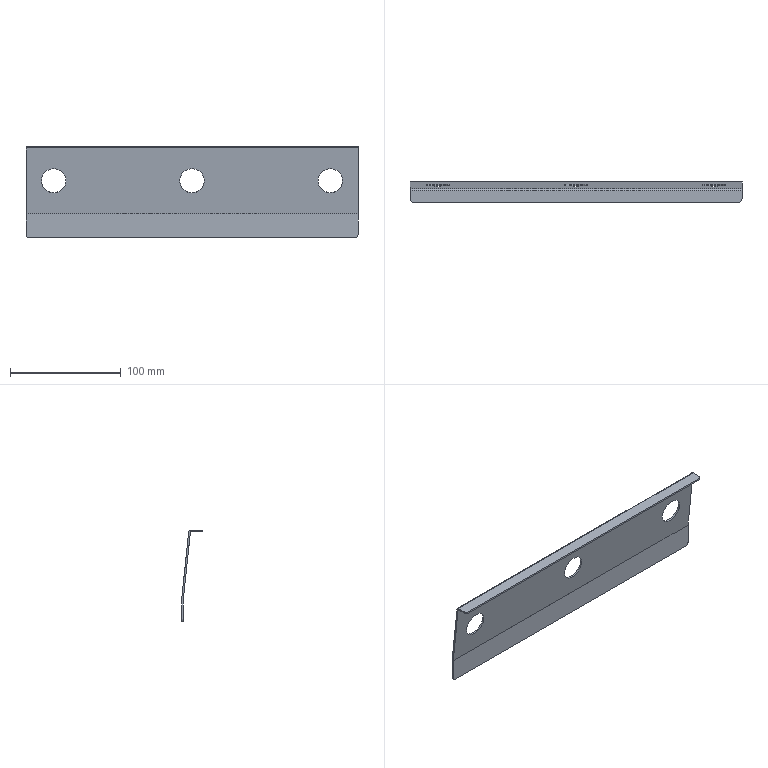Part | SolidWorks | features Fillet 1, FlatPattern 1, ICE 1, SMBaseFlange 1, SheetMetal 1 | 1 solid | 32 faces | box 300 x 18.411 x 83 mm | volume 40385 mm3 | plane 18 | cylinder 14 | commonest cylinder face diameters 22 x6 6 x4 0.5 x2 3.5 x2
STEP:
#1=CARTESIAN_POINT('',(125.,46.53,-10.476));
#2=VERTEX_POINT('',#1);
#3=CARTESIAN_POINT('',(125.,44.23,11.403));
#4=VERTEX_POINT('',#3);
#5=CARTESIAN_POINT('',(125.,45.38,0.4635));
#6=DIRECTION('',(0.,0.9945,0.1045));
#7=DIRECTION('',(0.,-0.1045,0.9945));
#8=AXIS2_PLACEMENT_3D('',#5,#6,#7);
#9=CIRCLE('',#8,11.);
#10=EDGE_CURVE('',#2,#4,#9,.T.);
#11=ORIENTED_EDGE('',*,*,#10,.F.);
#12=CARTESIAN_POINT('',(125.,48.022,-10.319));
#13=VERTEX_POINT('',#12);
#14=CARTESIAN_POINT('',(125.,38.076,-11.365));
#15=DIRECTION('',(0.,0.9945,0.1045));
#16=VECTOR('',#15,1000.);
#17=LINE('',#14,#16);
#18=EDGE_CURVE('',#2,#13,#17,.T.);
#19=ORIENTED_EDGE('',*,*,#18,.T.);
#20=CARTESIAN_POINT('',(125.,45.722,11.56));
#21=VERTEX_POINT('',#20);
#22=CARTESIAN_POINT('',(125.,46.872,0.6203));
#23=DIRECTION('',(0.,0.9945,0.1045));
#24=DIRECTION('',(0.,-0.1045,0.9945));
#25=AXIS2_PLACEMENT_3D('',#22,#23,#24);
#26=CIRCLE('',#25,11.);
#27=EDGE_CURVE('',#13,#21,#26,.T.);
#28=ORIENTED_EDGE('',*,*,#27,.T.);
#29=CARTESIAN_POINT('',(125.,35.777,10.515));
#30=DIRECTION('',(0.,0.9945,0.1045));
#31=VECTOR('',#30,1000.);
#32=LINE('',#29,#31);
#33=EDGE_CURVE('',#4,#21,#32,.T.);
#34=ORIENTED_EDGE('',*,*,#33,.F.);
#35=EDGE_LOOP('',(#11,#19,#28,#34));
#36=FACE_OUTER_BOUND('',#35,.T.);
#37=CARTESIAN_POINT('',(125.,36.927,-0.425));
#38=DIRECTION('',(0.,0.9945,0.1045));
#39=DIRECTION('',(0.,-0.1045,0.9945));
#40=AXIS2_PLACEMENT_3D('',#37,#38,#39);
#41=CYLINDRICAL_SURFACE('',#40,11.);
#42=ADVANCED_FACE('',(#36),#41,.F.);
#43=CARTESIAN_POINT('',(0.,46.53,-10.476));
#44=VERTEX_POINT('',#43);
#45=CARTESIAN_POINT('',(0.,44.23,11.403));
#46=VERTEX_POINT('',#45);
#47=CARTESIAN_POINT('',(0.,45.38,0.4635));
#48=DIRECTION('',(0.,0.9945,0.1045));
#49=DIRECTION('',(0.,-0.1045,0.9945));
#50=AXIS2_PLACEMENT_3D('',#47,#48,#49);
#51=CIRCLE('',#50,11.);
#52=EDGE_CURVE('',#44,#46,#51,.T.);
#53=ORIENTED_EDGE('',*,*,#52,.F.);
#54=CARTESIAN_POINT('',(0.,48.022,-10.319));
#55=VERTEX_POINT('',#54);
#56=CARTESIAN_POINT('',(0.,38.076,-11.365));
#57=DIRECTION('',(0.,0.9945,0.1045));
#58=VECTOR('',#57,1000.);
#59=LINE('',#56,#58);
#60=EDGE_CURVE('',#44,#55,#59,.T.);
#61=ORIENTED_EDGE('',*,*,#60,.T.);
#62=CARTESIAN_POINT('',(0.,45.722,11.56));
#63=VERTEX_POINT('',#62);
#64=CARTESIAN_POINT('',(0.,46.872,0.6203));
#65=DIRECTION('',(0.,0.9945,0.1045));
#66=DIRECTION('',(0.,-0.1045,0.9945));
#67=AXIS2_PLACEMENT_3D('',#64,#65,#66);
#68=CIRCLE('',#67,11.);
#69=EDGE_CURVE('',#55,#63,#68,.T.);
#70=ORIENTED_EDGE('',*,*,#69,.T.);
#71=CARTESIAN_POINT('',(0.,35.777,10.515));
#72=DIRECTION('',(0.,0.9945,0.1045));
#73=VECTOR('',#72,1000.);
#74=LINE('',#71,#73);
#75=EDGE_CURVE('',#46,#63,#74,.T.);
#76=ORIENTED_EDGE('',*,*,#75,.F.);
#77=EDGE_LOOP('',(#53,#61,#70,#76));
#78=FACE_OUTER_BOUND('',#77,.T.);
#79=CARTESIAN_POINT('',(0.,36.927,-0.425));
#80=DIRECTION('',(0.,0.9945,0.1045));
#81=DIRECTION('',(0.,-0.1045,0.9945));
#82=AXIS2_PLACEMENT_3D('',#79,#80,#81);
#83=CYLINDRICAL_SURFACE('',#82,11.);
#84=ADVANCED_FACE('',(#78),#83,.F.);
#85=CARTESIAN_POINT('',(-125.,46.53,-10.476));
#86=VERTEX_POINT('',#85);
#87=CARTESIAN_POINT('',(-125.,44.23,11.403));
#88=VERTEX_POINT('',#87);
#89=CARTESIAN_POINT('',(-125.,45.38,0.4635));
#90=DIRECTION('',(0.,0.9945,0.1045));
#91=DIRECTION('',(0.,-0.1045,0.9945));
#92=AXIS2_PLACEMENT_3D('',#89,#90,#91);
#93=CIRCLE('',#92,11.);
#94=EDGE_CURVE('',#86,#88,#93,.T.);
#95=ORIENTED_EDGE('',*,*,#94,.F.);
#96=CARTESIAN_POINT('',(-125.,48.022,-10.319));
#97=VERTEX_POINT('',#96);
#98=CARTESIAN_POINT('',(-125.,38.076,-11.365));
#99=DIRECTION('',(0.,0.9945,0.1045));
#100=VECTOR('',#99,1000.);
#101=LINE('',#98,#100);
#102=EDGE_CURVE('',#86,#97,#101,.T.);
#103=ORIENTED_EDGE('',*,*,#102,.T.);
#104=CARTESIAN_POINT('',(-125.,45.722,11.56));
#105=VERTEX_POINT('',#104);
#106=CARTESIAN_POINT('',(-125.,46.872,0.6203));
#107=DIRECTION('',(0.,0.9945,0.1045));
#108=DIRECTION('',(0.,0.1045,-0.9945));
#109=AXIS2_PLACEMENT_3D('',#106,#107,#108);
#110=CIRCLE('',#109,11.);
#111=EDGE_CURVE('',#97,#105,#110,.T.);
#112=ORIENTED_EDGE('',*,*,#111,.T.);
#113=CARTESIAN_POINT('',(-125.,35.777,10.515));
#114=DIRECTION('',(0.,0.9945,0.1045));
#115=VECTOR('',#114,1000.);
#116=LINE('',#113,#115);
#117=EDGE_CURVE('',#88,#105,#116,.T.);
#118=ORIENTED_EDGE('',*,*,#117,.F.);
#119=EDGE_LOOP('',(#95,#103,#112,#118));
#120=FACE_OUTER_BOUND('',#119,.T.);
#121=CARTESIAN_POINT('',(-125.,36.927,-0.425));
#122=DIRECTION('',(0.,0.9945,0.1045));
#123=DIRECTION('',(0.,-0.1045,0.9945));
#124=AXIS2_PLACEMENT_3D('',#121,#122,#123);
#125=CYLINDRICAL_SURFACE('',#124,11.);
#126=ADVANCED_FACE('',(#120),#125,.F.);
#127=CARTESIAN_POINT('',(150.,43.753,30.291));
#128=VERTEX_POINT('',#127);
#129=CARTESIAN_POINT('',(150.,42.262,30.134));
#130=VERTEX_POINT('',#129);
#131=CARTESIAN_POINT('',(150.,43.753,30.291));
#132=DIRECTION('',(0.,-0.9945,-0.1045));
#133=VECTOR('',#132,1000.);
#134=LINE('',#131,#133);
#135=EDGE_CURVE('',#128,#130,#134,.T.);
#136=ORIENTED_EDGE('',*,*,#135,.F.);
#137=CARTESIAN_POINT('',(150.,42.013,31.858));
#138=VERTEX_POINT('',#137);
#139=CARTESIAN_POINT('',(150.,42.013,30.108));
#140=DIRECTION('',(-1.,0.,0.));
#141=DIRECTION('',(0.,0.,-1.));
#142=AXIS2_PLACEMENT_3D('',#139,#140,#141);
#143=CIRCLE('',#142,1.75);
#144=EDGE_CURVE('',#138,#128,#143,.T.);
#145=ORIENTED_EDGE('',*,*,#144,.F.);
#146=CARTESIAN_POINT('',(150.,42.013,30.358));
#147=VERTEX_POINT('',#146);
#148=CARTESIAN_POINT('',(150.,42.013,30.358));
#149=DIRECTION('',(0.,0.,1.));
#150=VECTOR('',#149,1000.);
#151=LINE('',#148,#150);
#152=EDGE_CURVE('',#147,#138,#151,.T.);
#153=ORIENTED_EDGE('',*,*,#152,.F.);
#154=CARTESIAN_POINT('',(150.,42.013,30.108));
#155=DIRECTION('',(-1.,0.,0.));
#156=DIRECTION('',(0.,0.,-1.));
#157=AXIS2_PLACEMENT_3D('',#154,#155,#156);
#158=CIRCLE('',#157,0.25);
#159=EDGE_CURVE('',#147,#130,#158,.T.);
#160=ORIENTED_EDGE('',*,*,#159,.T.);
#161=EDGE_LOOP('',(#136,#145,#153,#160));
#162=FACE_OUTER_BOUND('',#161,.T.);
#163=CARTESIAN_POINT('',(150.,43.753,30.291));
#164=DIRECTION('',(1.,0.,0.));
#165=DIRECTION('',(0.,0.,-1.));
#166=AXIS2_PLACEMENT_3D('',#163,#164,#165);
#167=PLANE('',#166);
#168=ADVANCED_FACE('',(#162),#167,.T.);
#169=CARTESIAN_POINT('',(150.,49.99,-29.051));
#170=VERTEX_POINT('',#169);
#171=CARTESIAN_POINT('',(150.,43.589,31.858));
#172=DIRECTION('',(0.,0.1045,-0.9945));
#173=VECTOR('',#172,1000.);
#174=LINE('',#171,#173);
#175=EDGE_CURVE('',#128,#170,#174,.T.);
#176=ORIENTED_EDGE('',*,*,#175,.F.);
#177=ORIENTED_EDGE('',*,*,#135,.T.);
#178=CARTESIAN_POINT('',(150.,48.499,-29.207));
#179=VERTEX_POINT('',#178);
#180=CARTESIAN_POINT('',(150.,42.097,31.701));
#181=DIRECTION('',(0.,0.1045,-0.9945));
#182=VECTOR('',#181,1000.);
#183=LINE('',#180,#182);
#184=EDGE_CURVE('',#130,#179,#183,.T.);
#185=ORIENTED_EDGE('',*,*,#184,.T.);
#186=CARTESIAN_POINT('',(150.,48.499,-29.207));
#187=DIRECTION('',(0.,0.9945,0.1045));
#188=VECTOR('',#187,1000.);
#189=LINE('',#186,#188);
#190=EDGE_CURVE('',#179,#170,#189,.T.);
#191=ORIENTED_EDGE('',*,*,#190,.T.);
#192=EDGE_LOOP('',(#176,#177,#185,#191));
#193=FACE_OUTER_BOUND('',#192,.T.);
#194=CARTESIAN_POINT('',(150.,42.013,30.358));
#195=DIRECTION('',(1.,0.,0.));
#196=DIRECTION('',(0.,0.,-1.));
#197=AXIS2_PLACEMENT_3D('',#194,#195,#196);
#198=PLANE('',#197);
#199=ADVANCED_FACE('',(#193),#198,.T.);
#200=CARTESIAN_POINT('',(-150.,42.013,31.858));
#201=VERTEX_POINT('',#200);
#202=CARTESIAN_POINT('',(-150.,42.013,30.358));
#203=VERTEX_POINT('',#202);
#204=CARTESIAN_POINT('',(-150.,42.013,31.858));
#205=DIRECTION('',(0.,0.,-1.));
#206=VECTOR('',#205,1000.);
#207=LINE('',#204,#206);
#208=EDGE_CURVE('',#201,#203,#207,.T.);
#209=ORIENTED_EDGE('',*,*,#208,.F.);
#210=CARTESIAN_POINT('',(-150.,43.753,30.291));
#211=VERTEX_POINT('',#210);
#212=CARTESIAN_POINT('',(-150.,42.013,30.108));
#213=DIRECTION('',(-1.,0.,0.));
#214=DIRECTION('',(0.,0.,-1.));
#215=AXIS2_PLACEMENT_3D('',#212,#213,#214);
#216=CIRCLE('',#215,1.75);
#217=EDGE_CURVE('',#201,#211,#216,.T.);
#218=ORIENTED_EDGE('',*,*,#217,.T.);
#219=CARTESIAN_POINT('',(-150.,42.262,30.134));
#220=VERTEX_POINT('',#219);
#221=CARTESIAN_POINT('',(-150.,42.262,30.134));
#222=DIRECTION('',(0.,0.9945,0.1045));
#223=VECTOR('',#222,1000.);
#224=LINE('',#221,#223);
#225=EDGE_CURVE('',#220,#211,#224,.T.);
#226=ORIENTED_EDGE('',*,*,#225,.F.);
#227=CARTESIAN_POINT('',(-150.,42.013,30.108));
#228=DIRECTION('',(-1.,0.,0.));
#229=DIRECTION('',(0.,0.,-1.));
#230=AXIS2_PLACEMENT_3D('',#227,#228,#229);
#231=CIRCLE('',#230,0.25);
#232=EDGE_CURVE('',#203,#220,#231,.T.);
#233=ORIENTED_EDGE('',*,*,#232,.F.);
#234=EDGE_LOOP('',(#209,#218,#226,#233));
#235=FACE_OUTER_BOUND('',#234,.T.);
#236=CARTESIAN_POINT('',(-150.,42.013,31.858));
#237=DIRECTION('',(-1.,0.,0.));
#238=DIRECTION('',(0.,0.,1.));
#239=AXIS2_PLACEMENT_3D('',#236,#237,#238);
#240=PLANE('',#239);
#241=ADVANCED_FACE('',(#235),#240,.T.);
#242=CARTESIAN_POINT('',(-150.,34.589,30.358));
#243=VERTEX_POINT('',#242);
#244=CARTESIAN_POINT('',(-150.,31.589,30.358));
#245=DIRECTION('',(0.,1.,0.));
#246=VECTOR('',#245,1000.);
#247=LINE('',#244,#246);
#248=EDGE_CURVE('',#243,#203,#247,.T.);
#249=ORIENTED_EDGE('',*,*,#248,.F.);
#250=CARTESIAN_POINT('',(-150.,34.589,31.858));
#251=VERTEX_POINT('',#250);
#252=CARTESIAN_POINT('',(-150.,34.589,30.134));
#253=DIRECTION('',(0.,0.,1.));
#254=VECTOR('',#253,1000.);
#255=LINE('',#252,#254);
#256=EDGE_CURVE('',#243,#251,#255,.T.);
#257=ORIENTED_EDGE('',*,*,#256,.T.);
#258=CARTESIAN_POINT('',(-150.,31.589,31.858));
#259=DIRECTION('',(0.,1.,0.));
#260=VECTOR('',#259,1000.);
#261=LINE('',#258,#260);
#262=EDGE_CURVE('',#251,#201,#261,.T.);
#263=ORIENTED_EDGE('',*,*,#262,.T.);
#264=ORIENTED_EDGE('',*,*,#208,.T.);
#265=EDGE_LOOP('',(#249,#257,#263,#264));
#266=FACE_OUTER_BOUND('',#265,.T.);
#267=CARTESIAN_POINT('',(-150.,42.262,30.134));
#268=DIRECTION('',(-1.,0.,0.));
#269=DIRECTION('',(0.,0.,1.));
#270=AXIS2_PLACEMENT_3D('',#267,#268,#269);
#271=PLANE('',#270);
#272=ADVANCED_FACE('',(#266),#271,.T.);
#273=CARTESIAN_POINT('',(150.,50.,-29.233));
#274=VERTEX_POINT('',#273);
#275=CARTESIAN_POINT('',(150.,48.5,-29.233));
#276=VERTEX_POINT('',#275);
#277=CARTESIAN_POINT('',(150.,50.,-29.233));
#278=DIRECTION('',(0.,-1.,0.));
#279=VECTOR('',#278,1000.);
#280=LINE('',#277,#279);
#281=EDGE_CURVE('',#274,#276,#280,.T.);
#282=ORIENTED_EDGE('',*,*,#281,.F.);
#283=CARTESIAN_POINT('',(150.,48.25,-29.233));
#284=DIRECTION('',(-1.,0.,0.));
#285=DIRECTION('',(0.,0.,-1.));
#286=AXIS2_PLACEMENT_3D('',#283,#284,#285);
#287=CIRCLE('',#286,1.75);
#288=EDGE_CURVE('',#170,#274,#287,.T.);
#289=ORIENTED_EDGE('',*,*,#288,.F.);
#290=ORIENTED_EDGE('',*,*,#190,.F.);
#291=CARTESIAN_POINT('',(150.,48.25,-29.233));
#292=DIRECTION('',(-1.,0.,0.));
#293=DIRECTION('',(0.,0.,-1.));
#294=AXIS2_PLACEMENT_3D('',#291,#292,#293);
#295=CIRCLE('',#294,0.25);
#296=EDGE_CURVE('',#179,#276,#295,.T.);
#297=ORIENTED_EDGE('',*,*,#296,.T.);
#298=EDGE_LOOP('',(#282,#289,#290,#297));
#299=FACE_OUTER_BOUND('',#298,.T.);
#300=CARTESIAN_POINT('',(150.,50.,-29.233));
#301=DIRECTION('',(1.,0.,0.));
#302=DIRECTION('',(0.,0.,-1.));
#303=AXIS2_PLACEMENT_3D('',#300,#301,#302);
#304=PLANE('',#303);
#305=ADVANCED_FACE('',(#299),#304,.T.);
#306=CARTESIAN_POINT('',(150.,48.5,-48.142));
#307=VERTEX_POINT('',#306);
#308=CARTESIAN_POINT('',(150.,48.5,-29.142));
#309=DIRECTION('',(0.,0.,-1.));
#310=VECTOR('',#309,1000.);
#311=LINE('',#308,#310);
#312=EDGE_CURVE('',#276,#307,#311,.T.);
#313=ORIENTED_EDGE('',*,*,#312,.T.);
#314=CARTESIAN_POINT('',(150.,50.,-48.142));
#315=VERTEX_POINT('',#314);
#316=CARTESIAN_POINT('',(150.,48.499,-48.142));
#317=DIRECTION('',(0.,1.,0.));
#318=VECTOR('',#317,1000.);
#319=LINE('',#316,#318);
#320=EDGE_CURVE('',#307,#315,#319,.T.);
#321=ORIENTED_EDGE('',*,*,#320,.T.);
#322=CARTESIAN_POINT('',(150.,50.,-29.142));
#323=DIRECTION('',(0.,0.,-1.));
#324=VECTOR('',#323,1000.);
#325=LINE('',#322,#324);
#326=EDGE_CURVE('',#274,#315,#325,.T.);
#327=ORIENTED_EDGE('',*,*,#326,.F.);
#328=ORIENTED_EDGE('',*,*,#281,.T.);
#329=EDGE_LOOP('',(#313,#321,#327,#328));
#330=FACE_OUTER_BOUND('',#329,.T.);
#331=CARTESIAN_POINT('',(150.,48.499,-29.207));
#332=DIRECTION('',(1.,0.,0.));
#333=DIRECTION('',(0.,0.,-1.));
#334=AXIS2_PLACEMENT_3D('',#331,#332,#333);
#335=PLANE('',#334);
#336=ADVANCED_FACE('',(#330),#335,.T.);
#337=CARTESIAN_POINT('',(-150.,49.99,-29.051));
#338=VERTEX_POINT('',#337);
#339=CARTESIAN_POINT('',(-150.,48.499,-29.207));
#340=VERTEX_POINT('',#339);
#341=CARTESIAN_POINT('',(-150.,49.99,-29.051));
#342=DIRECTION('',(0.,-0.9945,-0.1045));
#343=VECTOR('',#342,1000.);
#344=LINE('',#341,#343);
#345=EDGE_CURVE('',#338,#340,#344,.T.);
#346=ORIENTED_EDGE('',*,*,#345,.F.);
#347=CARTESIAN_POINT('',(-150.,50.,-29.233));
#348=VERTEX_POINT('',#347);
#349=CARTESIAN_POINT('',(-150.,48.25,-29.233));
#350=DIRECTION('',(-1.,0.,0.));
#351=DIRECTION('',(0.,0.,-1.));
#352=AXIS2_PLACEMENT_3D('',#349,#350,#351);
#353=CIRCLE('',#352,1.75);
#354=EDGE_CURVE('',#338,#348,#353,.T.);
#355=ORIENTED_EDGE('',*,*,#354,.T.);
#356=CARTESIAN_POINT('',(-150.,48.5,-29.233));
#357=VERTEX_POINT('',#356);
#358=CARTESIAN_POINT('',(-150.,48.5,-29.233));
#359=DIRECTION('',(0.,1.,0.));
#360=VECTOR('',#359,1000.);
#361=LINE('',#358,#360);
#362=EDGE_CURVE('',#357,#348,#361,.T.);
#363=ORIENTED_EDGE('',*,*,#362,.F.);
#364=CARTESIAN_POINT('',(-150.,48.25,-29.233));
#365=DIRECTION('',(-1.,0.,0.));
#366=DIRECTION('',(0.,0.,-1.));
#367=AXIS2_PLACEMENT_3D('',#364,#365,#366);
#368=CIRCLE('',#367,0.25);
#369=EDGE_CURVE('',#340,#357,#368,.T.);
#370=ORIENTED_EDGE('',*,*,#369,.F.);
#371=EDGE_LOOP('',(#346,#355,#363,#370));
#372=FACE_OUTER_BOUND('',#371,.T.);
#373=CARTESIAN_POINT('',(-150.,49.99,-29.051));
#374=DIRECTION('',(-1.,0.,0.));
#375=DIRECTION('',(0.,0.,1.));
#376=AXIS2_PLACEMENT_3D('',#373,#374,#375);
#377=PLANE('',#376);
#378=ADVANCED_FACE('',(#372),#377,.T.);
#379=CARTESIAN_POINT('',(-150.,43.589,31.858));
#380=DIRECTION('',(0.,0.1045,-0.9945));
#381=VECTOR('',#380,1000.);
#382=LINE('',#379,#381);
#383=EDGE_CURVE('',#211,#338,#382,.T.);
#384=ORIENTED_EDGE('',*,*,#383,.T.);
#385=ORIENTED_EDGE('',*,*,#345,.T.);
#386=CARTESIAN_POINT('',(-150.,42.097,31.701));
#387=DIRECTION('',(0.,0.1045,-0.9945));
#388=VECTOR('',#387,1000.);
#389=LINE('',#386,#388);
#390=EDGE_CURVE('',#220,#340,#389,.T.);
#391=ORIENTED_EDGE('',*,*,#390,.F.);
#392=ORIENTED_EDGE('',*,*,#225,.T.);
#393=EDGE_LOOP('',(#384,#385,#391,#392));
#394=FACE_OUTER_BOUND('',#393,.T.);
#395=CARTESIAN_POINT('',(-150.,48.5,-29.233));
#396=DIRECTION('',(-1.,0.,0.));
#397=DIRECTION('',(0.,0.,1.));
#398=AXIS2_PLACEMENT_3D('',#395,#396,#397);
#399=PLANE('',#398);
#400=ADVANCED_FACE('',(#394),#399,.T.);
#401=CARTESIAN_POINT('',(-150.,48.5,-48.142));
#402=VERTEX_POINT('',#401);
#403=CARTESIAN_POINT('',(-150.,48.5,-29.142));
#404=DIRECTION('',(0.,0.,-1.));
#405=VECTOR('',#404,1000.);
#406=LINE('',#403,#405);
#407=EDGE_CURVE('',#357,#402,#406,.T.);
#408=ORIENTED_EDGE('',*,*,#407,.T.);
#409=CARTESIAN_POINT('',(-147.,48.5,-51.142));
#410=VERTEX_POINT('',#409);
#411=CARTESIAN_POINT('',(-147.,48.5,-48.142));
#412=DIRECTION('',(0.,-1.,0.));
#413=DIRECTION('',(0.,0.,1.));
#414=AXIS2_PLACEMENT_3D('',#411,#412,#413);
#415=CIRCLE('',#414,3.);
#416=EDGE_CURVE('',#402,#410,#415,.T.);
#417=ORIENTED_EDGE('',*,*,#416,.T.);
#418=CARTESIAN_POINT('',(147.,48.5,-51.142));
#419=VERTEX_POINT('',#418);
#420=CARTESIAN_POINT('',(150.,48.5,-51.142));
#421=DIRECTION('',(-1.,0.,0.));
#422=VECTOR('',#421,1000.);
#423=LINE('',#420,#422);
#424=EDGE_CURVE('',#419,#410,#423,.T.);
#425=ORIENTED_EDGE('',*,*,#424,.F.);
#426=CARTESIAN_POINT('',(147.,48.5,-48.142));
#427=DIRECTION('',(0.,-1.,0.));
#428=DIRECTION('',(0.,0.,1.));
#429=AXIS2_PLACEMENT_3D('',#426,#427,#428);
#430=CIRCLE('',#429,3.);
#431=EDGE_CURVE('',#419,#307,#430,.T.);
#432=ORIENTED_EDGE('',*,*,#431,.T.);
#433=ORIENTED_EDGE('',*,*,#312,.F.);
#434=CARTESIAN_POINT('',(150.,48.5,-29.233));
#435=DIRECTION('',(-1.,0.,0.));
#436=VECTOR('',#435,1000.);
#437=LINE('',#434,#436);
#438=EDGE_CURVE('',#276,#357,#437,.T.);
#439=ORIENTED_EDGE('',*,*,#438,.T.);
#440=EDGE_LOOP('',(#408,#417,#425,#432,#433,#439));
#441=FACE_OUTER_BOUND('',#440,.T.);
#442=CARTESIAN_POINT('',(150.,48.5,-29.142));
#443=DIRECTION('',(0.,1.,0.));
#444=DIRECTION('',(0.,0.,1.));
#445=AXIS2_PLACEMENT_3D('',#442,#443,#444);
#446=PLANE('',#445);
#447=ADVANCED_FACE('',(#441),#446,.F.);
#448=ORIENTED_EDGE('',*,*,#424,.T.);
#449=CARTESIAN_POINT('',(-147.,50.,-51.142));
#450=VERTEX_POINT('',#449);
#451=CARTESIAN_POINT('',(-147.,50.,-51.142));
#452=DIRECTION('',(0.,1.,0.));
#453=VECTOR('',#452,1000.);
#454=LINE('',#451,#453);
#455=EDGE_CURVE('',#410,#450,#454,.T.);
#456=ORIENTED_EDGE('',*,*,#455,.T.);
#457=CARTESIAN_POINT('',(147.,50.,-51.142));
#458=VERTEX_POINT('',#457);
#459=CARTESIAN_POINT('',(150.,50.,-51.142));
#460=DIRECTION('',(-1.,0.,0.));
#461=VECTOR('',#460,1000.);
#462=LINE('',#459,#461);
#463=EDGE_CURVE('',#458,#450,#462,.T.);
#464=ORIENTED_EDGE('',*,*,#463,.F.);
#465=CARTESIAN_POINT('',(147.,50.,-51.142));
#466=DIRECTION('',(0.,-1.,0.));
#467=VECTOR('',#466,1000.);
#468=LINE('',#465,#467);
#469=EDGE_CURVE('',#458,#419,#468,.T.);
#470=ORIENTED_EDGE('',*,*,#469,.T.);
#471=EDGE_LOOP('',(#448,#456,#464,#470));
#472=FACE_OUTER_BOUND('',#471,.T.);
#473=CARTESIAN_POINT('',(150.,50.,-51.142));
#474=DIRECTION('',(0.,0.,-1.));
#475=DIRECTION('',(-1.,0.,0.));
#476=AXIS2_PLACEMENT_3D('',#473,#474,#475);
#477=PLANE('',#476);
#478=ADVANCED_FACE('',(#472),#477,.T.);
#479=ORIENTED_EDGE('',*,*,#463,.T.);
#480=CARTESIAN_POINT('',(-150.,50.,-48.142));
#481=VERTEX_POINT('',#480);
#482=CARTESIAN_POINT('',(-147.,50.,-48.142));
#483=DIRECTION('',(0.,1.,0.));
#484=DIRECTION('',(0.,0.,1.));
#485=AXIS2_PLACEMENT_3D('',#482,#483,#484);
#486=CIRCLE('',#485,3.);
#487=EDGE_CURVE('',#450,#481,#486,.T.);
#488=ORIENTED_EDGE('',*,*,#487,.T.);
#489=CARTESIAN_POINT('',(-150.,50.,-29.142));
#490=DIRECTION('',(0.,0.,-1.));
#491=VECTOR('',#490,1000.);
#492=LINE('',#489,#491);
#493=EDGE_CURVE('',#348,#481,#492,.T.);
#494=ORIENTED_EDGE('',*,*,#493,.F.);
#495=CARTESIAN_POINT('',(150.,50.,-29.233));
#496=DIRECTION('',(-1.,0.,0.));
#497=VECTOR('',#496,1000.);
#498=LINE('',#495,#497);
#499=EDGE_CURVE('',#274,#348,#498,.T.);
#500=ORIENTED_EDGE('',*,*,#499,.F.);
#501=ORIENTED_EDGE('',*,*,#326,.T.);
#502=CARTESIAN_POINT('',(147.,50.,-48.142));
#503=DIRECTION('',(0.,1.,0.));
#504=DIRECTION('',(0.,0.,1.));
#505=AXIS2_PLACEMENT_3D('',#502,#503,#504);
#506=CIRCLE('',#505,3.);
#507=EDGE_CURVE('',#315,#458,#506,.T.);
#508=ORIENTED_EDGE('',*,*,#507,.T.);
#509=EDGE_LOOP('',(#479,#488,#494,#500,#501,#508));
#510=FACE_OUTER_BOUND('',#509,.T.);
#511=CARTESIAN_POINT('',(150.,50.,-29.142));
#512=DIRECTION('',(0.,1.,0.));
#513=DIRECTION('',(0.,0.,1.));
#514=AXIS2_PLACEMENT_3D('',#511,#512,#513);
#515=PLANE('',#514);
#516=ADVANCED_FACE('',(#510),#515,.T.);
#517=ORIENTED_EDGE('',*,*,#354,.F.);
#518=CARTESIAN_POINT('',(150.,49.99,-29.051));
#519=DIRECTION('',(-1.,0.,0.));
#520=VECTOR('',#519,1000.);
#521=LINE('',#518,#520);
#522=EDGE_CURVE('',#170,#338,#521,.T.);
#523=ORIENTED_EDGE('',*,*,#522,.F.);
#524=ORIENTED_EDGE('',*,*,#288,.T.);
#525=ORIENTED_EDGE('',*,*,#499,.T.);
#526=EDGE_LOOP('',(#517,#523,#524,#525));
#527=FACE_OUTER_BOUND('',#526,.T.);
#528=CARTESIAN_POINT('',(150.,48.25,-29.233));
#529=DIRECTION('',(-1.,0.,0.));
#530=DIRECTION('',(0.,0.,1.));
#531=AXIS2_PLACEMENT_3D('',#528,#529,#530);
#532=CYLINDRICAL_SURFACE('',#531,1.75);
#533=ADVANCED_FACE('',(#527),#532,.T.);
#534=CARTESIAN_POINT('',(125.,46.872,0.6203));
#535=DIRECTION('',(0.,0.9945,0.1045));
#536=DIRECTION('',(0.,-0.1045,0.9945));
#537=AXIS2_PLACEMENT_3D('',#534,#535,#536);
#538=CIRCLE('',#537,11.);
#539=EDGE_CURVE('',#21,#13,#538,.T.);
#540=ORIENTED_EDGE('',*,*,#539,.F.);
#541=ORIENTED_EDGE('',*,*,#27,.F.);
#542=EDGE_LOOP('',(#540,#541));
#543=FACE_BOUND('',#542,.T.);
#544=CARTESIAN_POINT('',(0.,46.872,0.6203));
#545=DIRECTION('',(0.,0.9945,0.1045));
#546=DIRECTION('',(0.,-0.1045,0.9945));
#547=AXIS2_PLACEMENT_3D('',#544,#545,#546);
#548=CIRCLE('',#547,11.);
#549=EDGE_CURVE('',#63,#55,#548,.T.);
#550=ORIENTED_EDGE('',*,*,#549,.F.);
#551=ORIENTED_EDGE('',*,*,#69,.F.);
#552=EDGE_LOOP('',(#550,#551));
#553=FACE_BOUND('',#552,.T.);
#554=CARTESIAN_POINT('',(-125.,46.872,0.6203));
#555=DIRECTION('',(0.,0.9945,0.1045));
#556=DIRECTION('',(0.,0.1045,-0.9945));
#557=AXIS2_PLACEMENT_3D('',#554,#555,#556);
#558=CIRCLE('',#557,11.);
#559=EDGE_CURVE('',#105,#97,#558,.T.);
#560=ORIENTED_EDGE('',*,*,#559,.F.);
#561=ORIENTED_EDGE('',*,*,#111,.F.);
#562=EDGE_LOOP('',(#560,#561));
#563=FACE_BOUND('',#562,.T.);
#564=ORIENTED_EDGE('',*,*,#383,.F.);
#565=CARTESIAN_POINT('',(150.,43.753,30.291));
#566=DIRECTION('',(-1.,0.,0.));
#567=VECTOR('',#566,1000.);
#568=LINE('',#565,#567);
#569=EDGE_CURVE('',#128,#211,#568,.T.);
#570=ORIENTED_EDGE('',*,*,#569,.F.);
#571=ORIENTED_EDGE('',*,*,#175,.T.);
#572=ORIENTED_EDGE('',*,*,#522,.T.);
#573=EDGE_LOOP('',(#564,#570,#571,#572));
#574=FACE_OUTER_BOUND('',#573,.T.);
#575=CARTESIAN_POINT('',(150.,43.589,31.858));
#576=DIRECTION('',(0.,0.9945,0.1045));
#577=DIRECTION('',(0.,-0.1045,0.9945));
#578=AXIS2_PLACEMENT_3D('',#575,#576,#577);
#579=PLANE('',#578);
#580=ADVANCED_FACE('',(#543,#553,#563,#574),#579,.T.);
#581=ORIENTED_EDGE('',*,*,#217,.F.);
#582=CARTESIAN_POINT('',(150.,42.013,31.858));
#583=DIRECTION('',(-1.,0.,0.));
#584=VECTOR('',#583,1000.);
#585=LINE('',#582,#584);
#586=EDGE_CURVE('',#138,#201,#585,.T.);
#587=ORIENTED_EDGE('',*,*,#586,.F.);
#588=ORIENTED_EDGE('',*,*,#144,.T.);
#589=ORIENTED_EDGE('',*,*,#569,.T.);
#590=EDGE_LOOP('',(#581,#587,#588,#589));
#591=FACE_OUTER_BOUND('',#590,.T.);
#592=CARTESIAN_POINT('',(150.,42.013,30.108));
#593=DIRECTION('',(-1.,0.,0.));
#594=DIRECTION('',(0.,0.,1.));
#595=AXIS2_PLACEMENT_3D('',#592,#593,#594);
#596=CYLINDRICAL_SURFACE('',#595,1.75);
#597=ADVANCED_FACE('',(#591),#596,.T.);
#598=ORIENTED_EDGE('',*,*,#262,.F.);
#599=CARTESIAN_POINT('',(-147.,31.589,31.858));
#600=VERTEX_POINT('',#599);
#601=CARTESIAN_POINT('',(-147.,34.589,31.858));
#602=DIRECTION('',(0.,0.,1.));
#603=DIRECTION('',(1.,0.,0.));
#604=AXIS2_PLACEMENT_3D('',#601,#602,#603);
#605=CIRCLE('',#604,3.);
#606=EDGE_CURVE('',#251,#600,#605,.T.);
#607=ORIENTED_EDGE('',*,*,#606,.T.);
#608=CARTESIAN_POINT('',(147.,31.589,31.858));
#609=VERTEX_POINT('',#608);
#610=CARTESIAN_POINT('',(150.,31.589,31.858));
#611=DIRECTION('',(-1.,0.,0.));
#612=VECTOR('',#611,1000.);
#613=LINE('',#610,#612);
#614=EDGE_CURVE('',#609,#600,#613,.T.);
#615=ORIENTED_EDGE('',*,*,#614,.F.);
#616=CARTESIAN_POINT('',(150.,34.589,31.858));
#617=VERTEX_POINT('',#616);
#618=CARTESIAN_POINT('',(147.,34.589,31.858));
#619=DIRECTION('',(0.,0.,1.));
#620=DIRECTION('',(1.,0.,0.));
#621=AXIS2_PLACEMENT_3D('',#618,#619,#620);
#622=CIRCLE('',#621,3.);
#623=EDGE_CURVE('',#609,#617,#622,.T.);
#624=ORIENTED_EDGE('',*,*,#623,.T.);
#625=CARTESIAN_POINT('',(150.,31.589,31.858));
#626=DIRECTION('',(0.,1.,0.));
#627=VECTOR('',#626,1000.);
#628=LINE('',#625,#627);
#629=EDGE_CURVE('',#617,#138,#628,.T.);
#630=ORIENTED_EDGE('',*,*,#629,.T.);
#631=ORIENTED_EDGE('',*,*,#586,.T.);
#632=EDGE_LOOP('',(#598,#607,#615,#624,#630,#631));
#633=FACE_OUTER_BOUND('',#632,.T.);
#634=CARTESIAN_POINT('',(150.,31.589,31.858));
#635=DIRECTION('',(0.,0.,1.));
#636=DIRECTION('',(1.,0.,0.));
#637=AXIS2_PLACEMENT_3D('',#634,#635,#636);
#638=PLANE('',#637);
#639=ADVANCED_FACE('',(#633),#638,.T.);
#640=ORIENTED_EDGE('',*,*,#614,.T.);
#641=CARTESIAN_POINT('',(-147.,31.589,30.358));
#642=VERTEX_POINT('',#641);
#643=CARTESIAN_POINT('',(-147.,31.589,30.358));
#644=DIRECTION('',(0.,0.,-1.));
#645=VECTOR('',#644,1000.);
#646=LINE('',#643,#645);
#647=EDGE_CURVE('',#600,#642,#646,.T.);
#648=ORIENTED_EDGE('',*,*,#647,.T.);
#649=CARTESIAN_POINT('',(147.,31.589,30.358));
#650=VERTEX_POINT('',#649);
#651=CARTESIAN_POINT('',(150.,31.589,30.358));
#652=DIRECTION('',(-1.,0.,0.));
#653=VECTOR('',#652,1000.);
#654=LINE('',#651,#653);
#655=EDGE_CURVE('',#650,#642,#654,.T.);
#656=ORIENTED_EDGE('',*,*,#655,.F.);
#657=CARTESIAN_POINT('',(147.,31.589,30.358));
#658=DIRECTION('',(0.,0.,1.));
#659=VECTOR('',#658,1000.);
#660=LINE('',#657,#659);
#661=EDGE_CURVE('',#650,#609,#660,.T.);
#662=ORIENTED_EDGE('',*,*,#661,.T.);
#663=EDGE_LOOP('',(#640,#648,#656,#662));
#664=FACE_OUTER_BOUND('',#663,.T.);
#665=CARTESIAN_POINT('',(150.,31.589,30.358));
#666=DIRECTION('',(0.,-1.,0.));
#667=DIRECTION('',(0.,0.,-1.));
#668=AXIS2_PLACEMENT_3D('',#665,#666,#667);
#669=PLANE('',#668);
#670=ADVANCED_FACE('',(#664),#669,.T.);
#671=ORIENTED_EDGE('',*,*,#655,.T.);
#672=CARTESIAN_POINT('',(-147.,34.589,30.358));
#673=DIRECTION('',(0.,0.,-1.));
#674=DIRECTION('',(1.,0.,0.));
#675=AXIS2_PLACEMENT_3D('',#672,#673,#674);
#676=CIRCLE('',#675,3.);
#677=EDGE_CURVE('',#642,#243,#676,.T.);
#678=ORIENTED_EDGE('',*,*,#677,.T.);
#679=ORIENTED_EDGE('',*,*,#248,.T.);
#680=CARTESIAN_POINT('',(150.,42.013,30.358));
#681=DIRECTION('',(-1.,0.,0.));
#682=VECTOR('',#681,1000.);
#683=LINE('',#680,#682);
#684=EDGE_CURVE('',#147,#203,#683,.T.);
#685=ORIENTED_EDGE('',*,*,#684,.F.);
#686=CARTESIAN_POINT('',(150.,34.589,30.358));
#687=VERTEX_POINT('',#686);
#688=CARTESIAN_POINT('',(150.,31.589,30.358));
#689=DIRECTION('',(0.,1.,0.));
#690=VECTOR('',#689,1000.);
#691=LINE('',#688,#690);
#692=EDGE_CURVE('',#687,#147,#691,.T.);
#693=ORIENTED_EDGE('',*,*,#692,.F.);
#694=CARTESIAN_POINT('',(147.,34.589,30.358));
#695=DIRECTION('',(0.,0.,-1.));
#696=DIRECTION('',(1.,0.,0.));
#697=AXIS2_PLACEMENT_3D('',#694,#695,#696);
#698=CIRCLE('',#697,3.);
#699=EDGE_CURVE('',#687,#650,#698,.T.);
#700=ORIENTED_EDGE('',*,*,#699,.T.);
#701=EDGE_LOOP('',(#671,#678,#679,#685,#693,#700));
#702=FACE_OUTER_BOUND('',#701,.T.);
#703=CARTESIAN_POINT('',(150.,31.589,30.358));
#704=DIRECTION('',(0.,0.,1.));
#705=DIRECTION('',(1.,0.,0.));
#706=AXIS2_PLACEMENT_3D('',#703,#704,#705);
#707=PLANE('',#706);
#708=ADVANCED_FACE('',(#702),#707,.F.);
#709=ORIENTED_EDGE('',*,*,#232,.T.);
#710=CARTESIAN_POINT('',(150.,42.262,30.134));
#711=DIRECTION('',(-1.,0.,0.));
#712=VECTOR('',#711,1000.);
#713=LINE('',#710,#712);
#714=EDGE_CURVE('',#130,#220,#713,.T.);
#715=ORIENTED_EDGE('',*,*,#714,.F.);
#716=ORIENTED_EDGE('',*,*,#159,.F.);
#717=ORIENTED_EDGE('',*,*,#684,.T.);
#718=EDGE_LOOP('',(#709,#715,#716,#717));
#719=FACE_OUTER_BOUND('',#718,.T.);
#720=CARTESIAN_POINT('',(150.,42.013,30.108));
#721=DIRECTION('',(-1.,0.,0.));
#722=DIRECTION('',(0.,0.,1.));
#723=AXIS2_PLACEMENT_3D('',#720,#721,#722);
#724=CYLINDRICAL_SURFACE('',#723,0.25);
#725=ADVANCED_FACE('',(#719),#724,.F.);
#726=CARTESIAN_POINT('',(125.,45.38,0.4635));
#727=DIRECTION('',(0.,0.9945,0.1045));
#728=DIRECTION('',(0.,-0.1045,0.9945));
#729=AXIS2_PLACEMENT_3D('',#726,#727,#728);
#730=CIRCLE('',#729,11.);
#731=EDGE_CURVE('',#4,#2,#730,.T.);
#732=ORIENTED_EDGE('',*,*,#731,.T.);
#733=ORIENTED_EDGE('',*,*,#10,.T.);
#734=EDGE_LOOP('',(#732,#733));
#735=FACE_BOUND('',#734,.T.);
#736=CARTESIAN_POINT('',(0.,45.38,0.4635));
#737=DIRECTION('',(0.,0.9945,0.1045));
#738=DIRECTION('',(0.,-0.1045,0.9945));
#739=AXIS2_PLACEMENT_3D('',#736,#737,#738);
#740=CIRCLE('',#739,11.);
#741=EDGE_CURVE('',#46,#44,#740,.T.);
#742=ORIENTED_EDGE('',*,*,#741,.T.);
#743=ORIENTED_EDGE('',*,*,#52,.T.);
#744=EDGE_LOOP('',(#742,#743));
#745=FACE_BOUND('',#744,.T.);
#746=CARTESIAN_POINT('',(-125.,45.38,0.4635));
#747=DIRECTION('',(0.,0.9945,0.1045));
#748=DIRECTION('',(0.,-0.1045,0.9945));
#749=AXIS2_PLACEMENT_3D('',#746,#747,#748);
#750=CIRCLE('',#749,11.);
#751=EDGE_CURVE('',#88,#86,#750,.T.);
#752=ORIENTED_EDGE('',*,*,#751,.T.);
#753=ORIENTED_EDGE('',*,*,#94,.T.);
#754=EDGE_LOOP('',(#752,#753));
#755=FACE_BOUND('',#754,.T.);
#756=ORIENTED_EDGE('',*,*,#390,.T.);
#757=CARTESIAN_POINT('',(150.,48.499,-29.207));
#758=DIRECTION('',(-1.,0.,0.));
#759=VECTOR('',#758,1000.);
#760=LINE('',#757,#759);
#761=EDGE_CURVE('',#179,#340,#760,.T.);
#762=ORIENTED_EDGE('',*,*,#761,.F.);
#763=ORIENTED_EDGE('',*,*,#184,.F.);
#764=ORIENTED_EDGE('',*,*,#714,.T.);
#765=EDGE_LOOP('',(#756,#762,#763,#764));
#766=FACE_OUTER_BOUND('',#765,.T.);
#767=CARTESIAN_POINT('',(150.,42.097,31.701));
#768=DIRECTION('',(0.,0.9945,0.1045));
#769=DIRECTION('',(0.,-0.1045,0.9945));
#770=AXIS2_PLACEMENT_3D('',#767,#768,#769);
#771=PLANE('',#770);
#772=ADVANCED_FACE('',(#735,#745,#755,#766),#771,.F.);
#773=ORIENTED_EDGE('',*,*,#369,.T.);
#774=ORIENTED_EDGE('',*,*,#438,.F.);
#775=ORIENTED_EDGE('',*,*,#296,.F.);
#776=ORIENTED_EDGE('',*,*,#761,.T.);
#777=EDGE_LOOP('',(#773,#774,#775,#776));
#778=FACE_OUTER_BOUND('',#777,.T.);
#779=CARTESIAN_POINT('',(150.,48.25,-29.233));
#780=DIRECTION('',(-1.,0.,0.));
#781=DIRECTION('',(0.,0.,1.));
#782=AXIS2_PLACEMENT_3D('',#779,#780,#781);
#783=CYLINDRICAL_SURFACE('',#782,0.25);
#784=ADVANCED_FACE('',(#778),#783,.F.);
#785=ORIENTED_EDGE('',*,*,#629,.F.);
#786=CARTESIAN_POINT('',(150.,34.589,-29.233));
#787=DIRECTION('',(0.,0.,-1.));
#788=VECTOR('',#787,1000.);
#789=LINE('',#786,#788);
#790=EDGE_CURVE('',#617,#687,#789,.T.);
#791=ORIENTED_EDGE('',*,*,#790,.T.);
#792=ORIENTED_EDGE('',*,*,#692,.T.);
#793=ORIENTED_EDGE('',*,*,#152,.T.);
#794=EDGE_LOOP('',(#785,#791,#792,#793));
#795=FACE_OUTER_BOUND('',#794,.T.);
#796=CARTESIAN_POINT('',(150.,48.25,-29.233));
#797=DIRECTION('',(1.,0.,0.));
#798=DIRECTION('',(0.,0.,-1.));
#799=AXIS2_PLACEMENT_3D('',#796,#797,#798);
#800=PLANE('',#799);
#801=ADVANCED_FACE('',(#795),#800,.T.);
#802=ORIENTED_EDGE('',*,*,#493,.T.);
#803=CARTESIAN_POINT('',(-150.,48.5,-48.142));
#804=DIRECTION('',(0.,-1.,0.));
#805=VECTOR('',#804,1000.);
#806=LINE('',#803,#805);
#807=EDGE_CURVE('',#481,#402,#806,.T.);
#808=ORIENTED_EDGE('',*,*,#807,.T.);
#809=ORIENTED_EDGE('',*,*,#407,.F.);
#810=ORIENTED_EDGE('',*,*,#362,.T.);
#811=EDGE_LOOP('',(#802,#808,#809,#810));
#812=FACE_OUTER_BOUND('',#811,.T.);
#813=CARTESIAN_POINT('',(-150.,48.25,-29.233));
#814=DIRECTION('',(1.,0.,0.));
#815=DIRECTION('',(0.,0.,-1.));
#816=AXIS2_PLACEMENT_3D('',#813,#814,#815);
#817=PLANE('',#816);
#818=ADVANCED_FACE('',(#812),#817,.F.);
#819=ORIENTED_EDGE('',*,*,#677,.F.);
#820=ORIENTED_EDGE('',*,*,#647,.F.);
#821=ORIENTED_EDGE('',*,*,#606,.F.);
#822=ORIENTED_EDGE('',*,*,#256,.F.);
#823=EDGE_LOOP('',(#819,#820,#821,#822));
#824=FACE_OUTER_BOUND('',#823,.T.);
#825=CARTESIAN_POINT('',(-147.,34.589,30.134));
#826=DIRECTION('',(0.,0.,1.));
#827=DIRECTION('',(1.,0.,0.));
#828=AXIS2_PLACEMENT_3D('',#825,#826,#827);
#829=CYLINDRICAL_SURFACE('',#828,3.);
#830=ADVANCED_FACE('',(#824),#829,.T.);
#831=ORIENTED_EDGE('',*,*,#487,.F.);
#832=ORIENTED_EDGE('',*,*,#455,.F.);
#833=ORIENTED_EDGE('',*,*,#416,.F.);
#834=ORIENTED_EDGE('',*,*,#807,.F.);
#835=EDGE_LOOP('',(#831,#832,#833,#834));
#836=FACE_OUTER_BOUND('',#835,.T.);
#837=CARTESIAN_POINT('',(-147.,48.25,-48.142));
#838=DIRECTION('',(0.,1.,0.));
#839=DIRECTION('',(0.,0.,1.));
#840=AXIS2_PLACEMENT_3D('',#837,#838,#839);
#841=CYLINDRICAL_SURFACE('',#840,3.);
#842=ADVANCED_FACE('',(#836),#841,.T.);
#843=ORIENTED_EDGE('',*,*,#507,.F.);
#844=ORIENTED_EDGE('',*,*,#320,.F.);
#845=ORIENTED_EDGE('',*,*,#431,.F.);
#846=ORIENTED_EDGE('',*,*,#469,.F.);
#847=EDGE_LOOP('',(#843,#844,#845,#846));
#848=FACE_OUTER_BOUND('',#847,.T.);
#849=CARTESIAN_POINT('',(147.,50.,-48.142));
#850=DIRECTION('',(0.,-1.,0.));
#851=DIRECTION('',(0.,0.,-1.));
#852=AXIS2_PLACEMENT_3D('',#849,#850,#851);
#853=CYLINDRICAL_SURFACE('',#852,3.);
#854=ADVANCED_FACE('',(#848),#853,.T.);
#855=ORIENTED_EDGE('',*,*,#699,.F.);
#856=ORIENTED_EDGE('',*,*,#790,.F.);
#857=ORIENTED_EDGE('',*,*,#623,.F.);
#858=ORIENTED_EDGE('',*,*,#661,.F.);
#859=EDGE_LOOP('',(#855,#856,#857,#858));
#860=FACE_OUTER_BOUND('',#859,.T.);
#861=CARTESIAN_POINT('',(147.,34.589,30.358));
#862=DIRECTION('',(0.,0.,1.));
#863=DIRECTION('',(1.,0.,0.));
#864=AXIS2_PLACEMENT_3D('',#861,#862,#863);
#865=CYLINDRICAL_SURFACE('',#864,3.);
#866=ADVANCED_FACE('',(#860),#865,.T.);
#867=ORIENTED_EDGE('',*,*,#102,.F.);
#868=ORIENTED_EDGE('',*,*,#751,.F.);
#869=ORIENTED_EDGE('',*,*,#117,.T.);
#870=ORIENTED_EDGE('',*,*,#559,.T.);
#871=EDGE_LOOP('',(#867,#868,#869,#870));
#872=FACE_OUTER_BOUND('',#871,.T.);
#873=CARTESIAN_POINT('',(-125.,36.927,-0.425));
#874=DIRECTION('',(0.,0.9945,0.1045));
#875=DIRECTION('',(0.,-0.1045,0.9945));
#876=AXIS2_PLACEMENT_3D('',#873,#874,#875);
#877=CYLINDRICAL_SURFACE('',#876,11.);
#878=ADVANCED_FACE('',(#872),#877,.F.);
#879=ORIENTED_EDGE('',*,*,#60,.F.);
#880=ORIENTED_EDGE('',*,*,#741,.F.);
#881=ORIENTED_EDGE('',*,*,#75,.T.);
#882=ORIENTED_EDGE('',*,*,#549,.T.);
#883=EDGE_LOOP('',(#879,#880,#881,#882));
#884=FACE_OUTER_BOUND('',#883,.T.);
#885=CARTESIAN_POINT('',(0.,36.927,-0.425));
#886=DIRECTION('',(0.,0.9945,0.1045));
#887=DIRECTION('',(0.,-0.1045,0.9945));
#888=AXIS2_PLACEMENT_3D('',#885,#886,#887);
#889=CYLINDRICAL_SURFACE('',#888,11.);
#890=ADVANCED_FACE('',(#884),#889,.F.);
#891=ORIENTED_EDGE('',*,*,#18,.F.);
#892=ORIENTED_EDGE('',*,*,#731,.F.);
#893=ORIENTED_EDGE('',*,*,#33,.T.);
#894=ORIENTED_EDGE('',*,*,#539,.T.);
#895=EDGE_LOOP('',(#891,#892,#893,#894));
#896=FACE_OUTER_BOUND('',#895,.T.);
#897=CARTESIAN_POINT('',(125.,36.927,-0.425));
#898=DIRECTION('',(0.,0.9945,0.1045));
#899=DIRECTION('',(0.,-0.1045,0.9945));
#900=AXIS2_PLACEMENT_3D('',#897,#898,#899);
#901=CYLINDRICAL_SURFACE('',#900,11.);
#902=ADVANCED_FACE('',(#896),#901,.F.);
#903=CLOSED_SHELL('',(#42,#84,#126,#168,#199,#241,#272,#305,#336,#378,#400,#447,#478,#516,#533,#580,#597,#639,#670,#708,#725,#772,#784,#801,#818,#830,#842,#854,#866,#878,#890,#902));
#904=MANIFOLD_SOLID_BREP('',#903);
#905=CARTESIAN_POINT('',(0.,0.,0.));
#906=DIRECTION('',(0.,0.,1.));
#907=DIRECTION('',(1.,0.,0.));
#908=AXIS2_PLACEMENT_3D('',#905,#906,#907);
#909=(LENGTH_UNIT()NAMED_UNIT(*)SI_UNIT(.MILLI.,.METRE.));
#910=UNCERTAINTY_MEASURE_WITH_UNIT(LENGTH_MEASURE(0.00001),#909,'','');
#911=(NAMED_UNIT(*)PLANE_ANGLE_UNIT()SI_UNIT($,.RADIAN.));
#912=(NAMED_UNIT(*)SI_UNIT($,.STERADIAN.)SOLID_ANGLE_UNIT());
#913=(GEOMETRIC_REPRESENTATION_CONTEXT(3)GLOBAL_UNCERTAINTY_ASSIGNED_CONTEXT((#910))GLOBAL_UNIT_ASSIGNED_CONTEXT((#909,#911,#912))REPRESENTATION_CONTEXT('',''));
#914=ADVANCED_BREP_SHAPE_REPRESENTATION('',(#904,#908),#913);